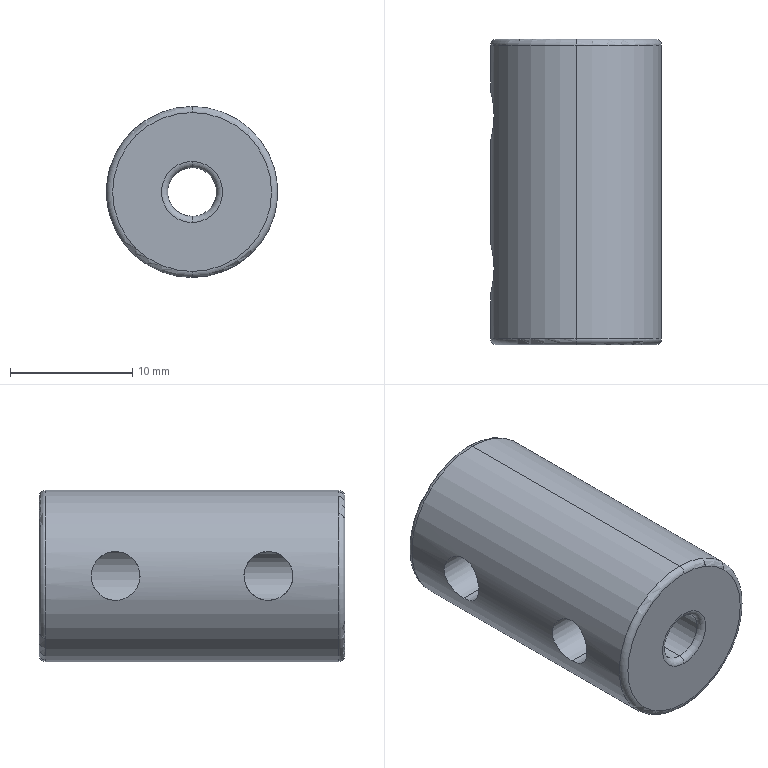Part | STEP file | 55 rigid coupling | 1 solid | 22 faces | box 14 x 25 x 14 mm | volume 3316 mm3 | cylinder 11 | torus 8 | plane 3 | commonest cylinder face diameters 4 x7 5 x2 14 x2